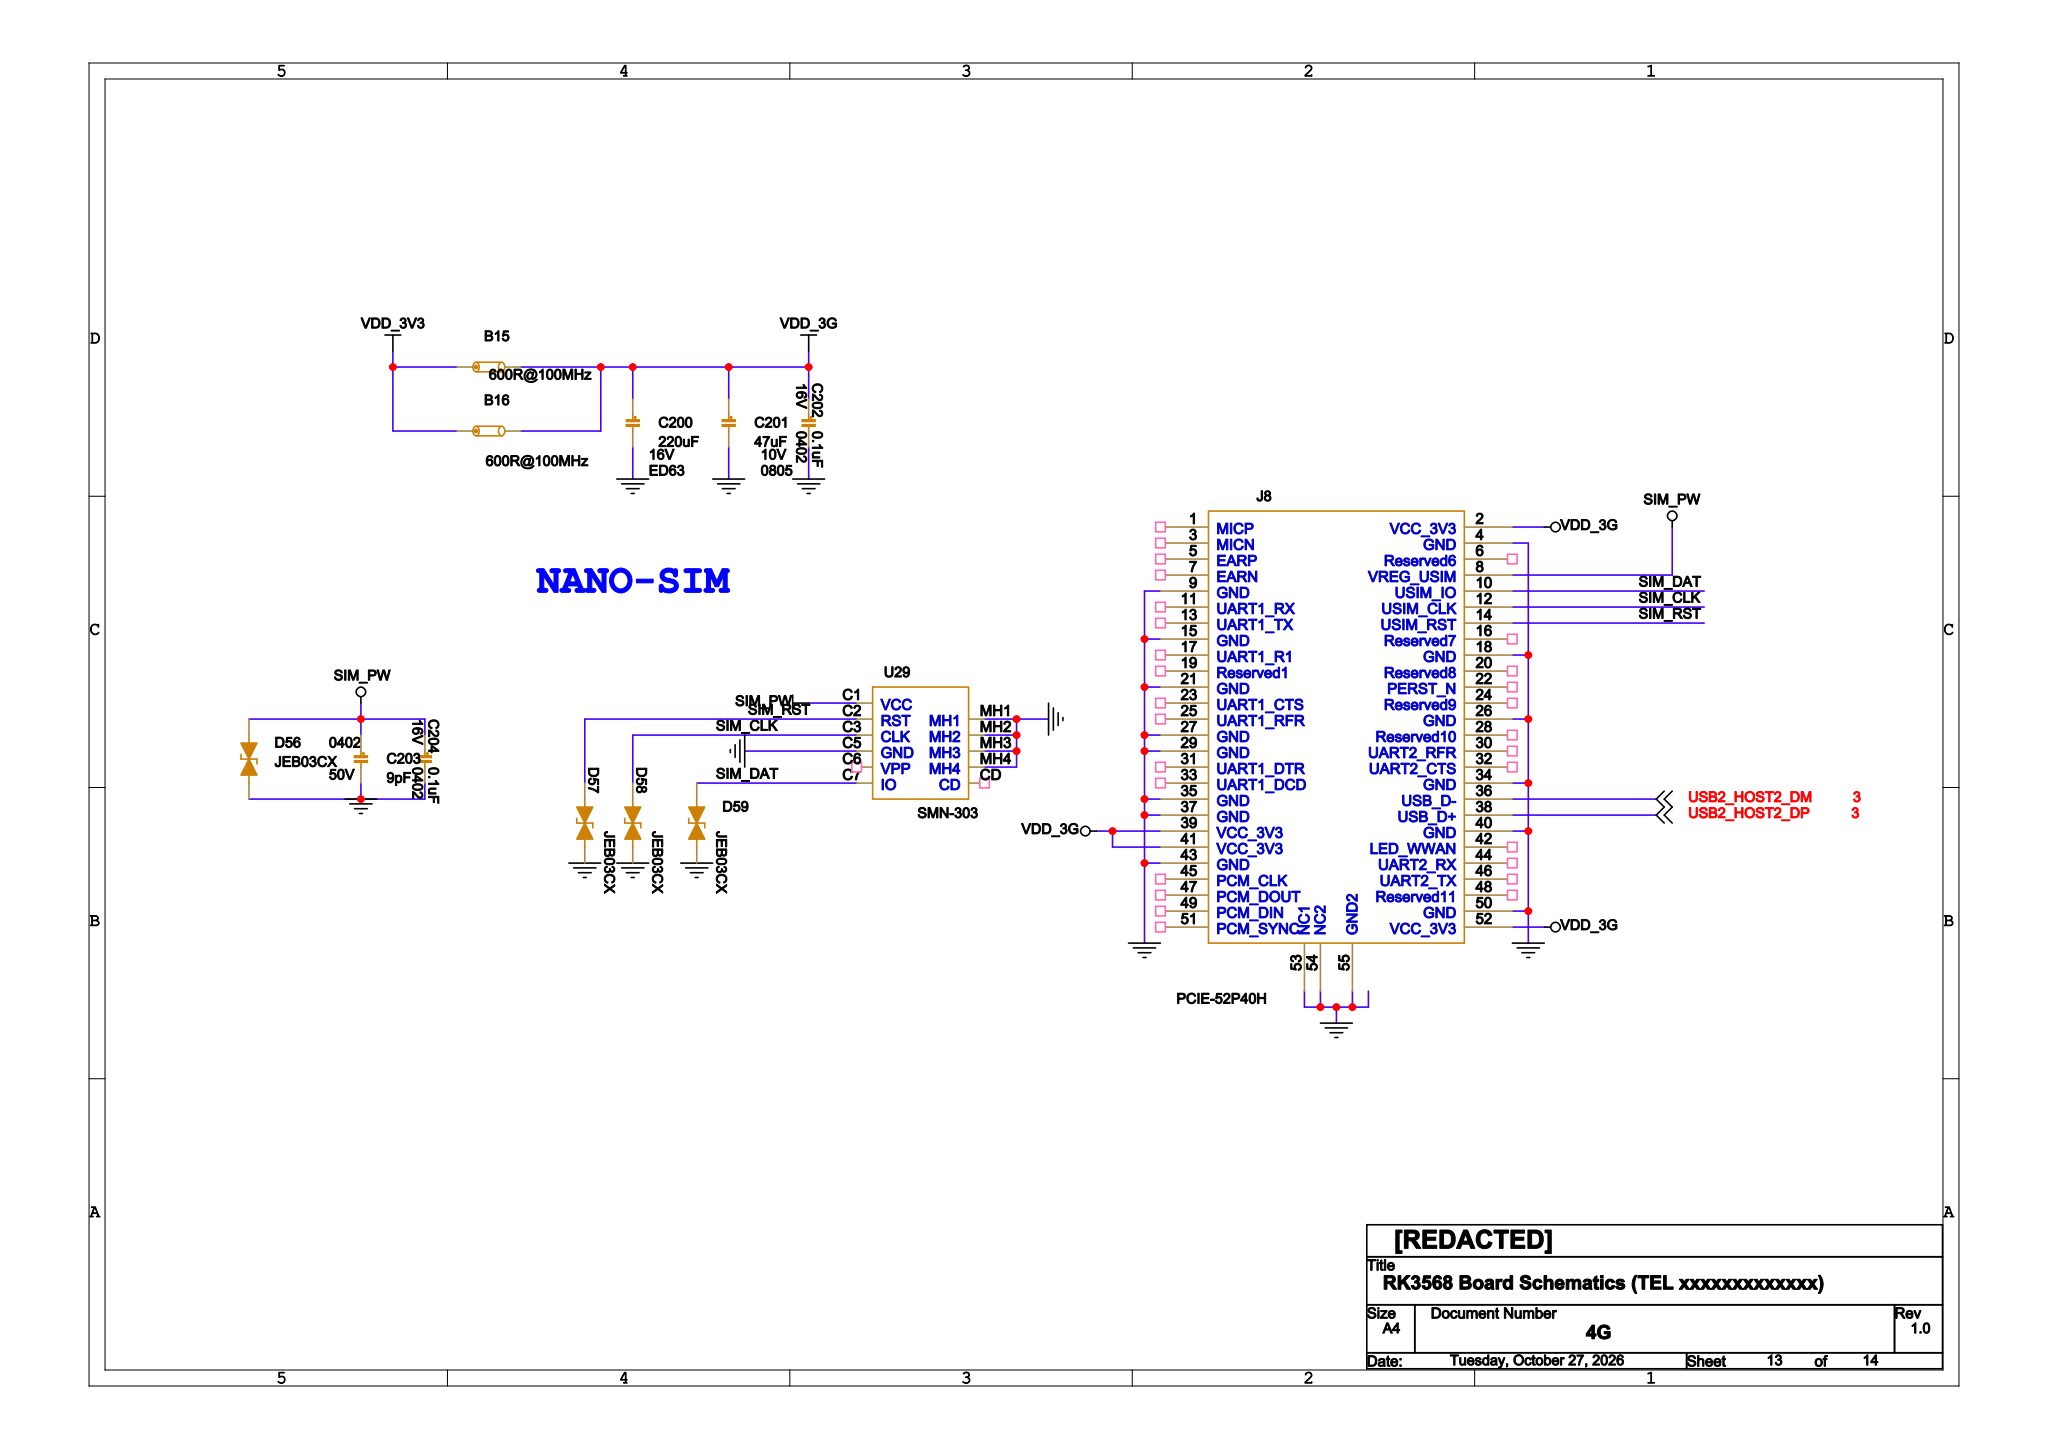Circuit board | Cadence Allegro | 669 parts | 581 nets | one sheet of the schematic
Parts on this sheet (reference | value | footprint):
B15 | 600R@100MHz | R0805
B16 | 600R@100MHz | R0805
C200 | 220uF | ED63
C201 | 47uF | C0805
C202 | 0.1uF | C0402
C204 | 0.1uF | C0402
D56 | JEB03CX | SOD323
D57 | JEB03CX | SOD323
D58 | JEB03CX | SOD323
D59 | JEB03CX | SOD323
J8 | PCIE-52P40H | MINI-PCIE-SMD
U29 | SMN-303 | MICRO_SIM_SMN_303
Nets of these parts (net: part-pin ...):
GND: C200-2 C201-2 C202-2 C204-2 D56-1 D57-1 D58-1 D59-1 U29-C5 U29-MH1 U29-MH2 U29-MH3 U29-MH4 J8-4 J8-9 J8-15 J8-18 J8-21 J8-26 J8-27 J8-29 J8-34 J8-35 J8-37 J8-40 J8-43 J8-50 J8-53 J8-54 J8-55
VCC3V3_SYS: B15-1 B16-1
VDD_3G: B15-2 B16-2 C200-1 C201-1 C202-1 J8-2 J8-39 J8-41 J8-52
SIM_PW: C204-1 D56-2 U29-C1 J8-8
SIM_RST: D57-2 U29-C2 J8-14
SIM_CLK: D58-2 U29-C3
SIM_DAT: D59-2 U29-C7 J8-10
USB2_HOST2_DP: J8-38
USB2_HOST2_DM: J8-36